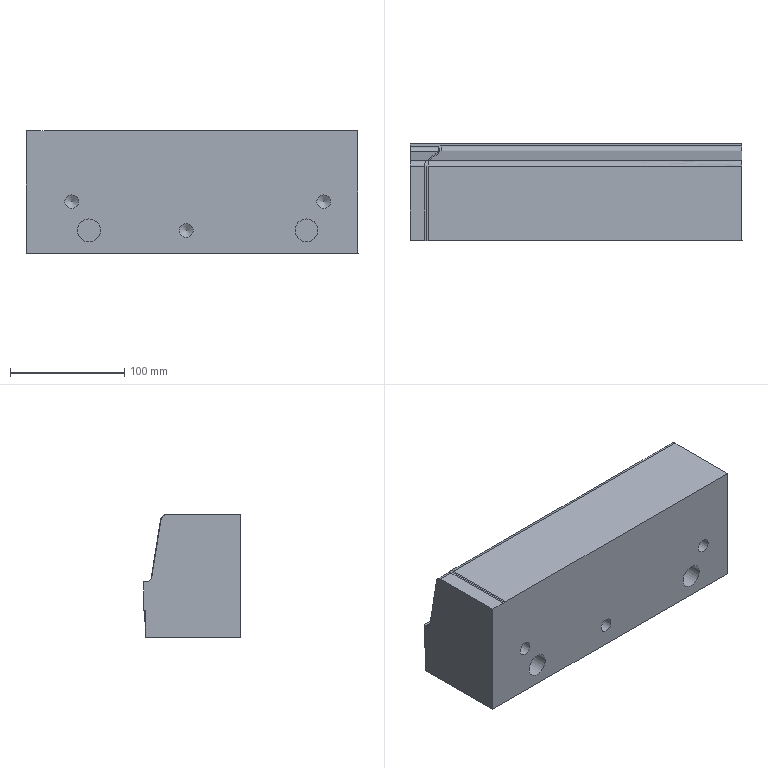Part | NX | features solid 2 | 1 solid | 33 faces | box 290 x 84.721 x 107.133 mm | volume 2405435 mm3 | plane 12 | cylinder 10 | spline 8 | cone 3 | commonest cylinder face diameters 12 x5 10 x3 20 x2
STEP:
#1=CARTESIAN_POINT('',(-215.,-160.,-50.));
#2=VERTEX_POINT('',#1);
#3=CARTESIAN_POINT('',(75.,-160.,-50.));
#4=VERTEX_POINT('',#3);
#5=CARTESIAN_POINT('',(-571.479,-160.,-50.));
#6=DIRECTION('',(1.,0.,0.));
#7=VECTOR('',#6,1000.);
#8=LINE('',#5,#7);
#9=EDGE_CURVE('',#2,#4,#8,.T.);
#10=ORIENTED_EDGE('',*,*,#9,.F.);
#11=CARTESIAN_POINT('',(-215.,-77.115,-50.));
#12=VERTEX_POINT('',#11);
#13=CARTESIAN_POINT('',(-215.,-74.471,-50.));
#14=DIRECTION('',(0.,1.,0.));
#15=VECTOR('',#14,1000.);
#16=LINE('',#13,#15);
#17=EDGE_CURVE('',#2,#12,#16,.T.);
#18=ORIENTED_EDGE('',*,*,#17,.T.);
#19=CARTESIAN_POINT('',(75.,-76.708,-50.));
#20=VERTEX_POINT('',#19);
#21=CARTESIAN_POINT('',(-215.,-77.115,-50.));
#22=CARTESIAN_POINT('',(-211.979,-77.116,-50.));
#23=CARTESIAN_POINT('',(-207.448,-77.118,-50.));
#24=CARTESIAN_POINT('',(-201.406,-77.119,-50.));
#25=CARTESIAN_POINT('',(-197.63,-77.126,-50.));
#26=CARTESIAN_POINT('',(-194.609,-77.116,-50.));
#27=CARTESIAN_POINT('',(-192.344,-77.15,-50.));
#28=CARTESIAN_POINT('',(-190.078,-77.04,-50.));
#29=CARTESIAN_POINT('',(-187.813,-76.65,-50.));
#30=CARTESIAN_POINT('',(-185.547,-76.717,-50.));
#31=CARTESIAN_POINT('',(-182.527,-76.699,-50.));
#32=CARTESIAN_POINT('',(-177.24,-76.699,-50.));
#33=CARTESIAN_POINT('',(-169.688,-76.703,-50.));
#34=CARTESIAN_POINT('',(-157.605,-76.713,-50.));
#35=CARTESIAN_POINT('',(-136.459,-76.708,-50.));
#36=CARTESIAN_POINT('',(-106.25,-76.699,-50.));
#37=CARTESIAN_POINT('',(-57.917,-76.699,-50.));
#38=CARTESIAN_POINT('',(2.5,-76.706,-50.));
#39=CARTESIAN_POINT('',(50.833,-76.708,-50.));
#40=CARTESIAN_POINT('',(75.,-76.708,-50.));
#41=B_SPLINE_CURVE_WITH_KNOTS('',3,(#21,#22,#23,#24,#25,#26,#27,#28,#29,#30,#31,#32,#33,#34,#35,#36,#37,#38,#39,#40),.UNSPECIFIED.,.F.,.F.,(4,1,1,1,1,1,1,1,1,1,1,1,1,1,1,1,1,4),(0.1494,0.1584,0.163,0.1675,0.1698,0.172,0.1743,0.1766,0.1788,0.1811,0.1856,0.1947,0.2037,0.2219,0.2581,0.2944,0.3669,0.4394),.UNSPECIFIED.);
#42=EDGE_CURVE('',#12,#20,#41,.T.);
#43=ORIENTED_EDGE('',*,*,#42,.T.);
#44=CARTESIAN_POINT('',(75.,-159.,-50.));
#45=DIRECTION('',(0.,1.,0.));
#46=VECTOR('',#45,1000.);
#47=LINE('',#44,#46);
#48=EDGE_CURVE('',#4,#20,#47,.T.);
#49=ORIENTED_EDGE('',*,*,#48,.F.);
#50=EDGE_LOOP('',(#10,#18,#43,#49));
#51=FACE_BOUND('',#50,.T.);
#52=CARTESIAN_POINT('',(-571.479,-74.471,-50.));
#53=DIRECTION('',(0.,0.,-1.));
#54=DIRECTION('',(-1.,0.,0.));
#55=AXIS2_PLACEMENT_3D('',#52,#53,#54);
#56=PLANE('',#55);
#57=ADVANCED_FACE('',(#51),#56,.T.);
#58=ORIENTED_EDGE('',*,*,#42,.F.);
#59=CARTESIAN_POINT('',(-215.,-76.915,-26.496));
#60=VERTEX_POINT('',#59);
#61=CARTESIAN_POINT('',(-215.,-77.015,-38.265));
#62=DIRECTION('',(0.,-0.008536,-1.));
#63=VECTOR('',#62,1000.);
#64=LINE('',#61,#63);
#65=EDGE_CURVE('',#12,#60,#64,.F.);
#66=ORIENTED_EDGE('',*,*,#65,.T.);
#67=CARTESIAN_POINT('',(75.,-76.507,-26.5));
#68=VERTEX_POINT('',#67);
#69=CARTESIAN_POINT('',(-215.,-76.915,-26.496));
#70=CARTESIAN_POINT('',(-211.979,-76.915,-26.496));
#71=CARTESIAN_POINT('',(-207.448,-76.918,-26.496));
#72=CARTESIAN_POINT('',(-201.406,-76.918,-26.496));
#73=CARTESIAN_POINT('',(-197.63,-76.925,-26.496));
#74=CARTESIAN_POINT('',(-194.609,-76.916,-26.496));
#75=CARTESIAN_POINT('',(-192.344,-76.949,-26.496));
#76=CARTESIAN_POINT('',(-190.078,-76.839,-26.497));
#77=CARTESIAN_POINT('',(-187.813,-76.449,-26.5));
#78=CARTESIAN_POINT('',(-185.547,-76.516,-26.499));
#79=CARTESIAN_POINT('',(-182.527,-76.499,-26.5));
#80=CARTESIAN_POINT('',(-177.24,-76.499,-26.5));
#81=CARTESIAN_POINT('',(-169.688,-76.502,-26.5));
#82=CARTESIAN_POINT('',(-157.605,-76.512,-26.5));
#83=CARTESIAN_POINT('',(-136.459,-76.507,-26.5));
#84=CARTESIAN_POINT('',(-106.25,-76.499,-26.5));
#85=CARTESIAN_POINT('',(-57.917,-76.498,-26.5));
#86=CARTESIAN_POINT('',(2.5,-76.505,-26.5));
#87=CARTESIAN_POINT('',(50.833,-76.507,-26.5));
#88=CARTESIAN_POINT('',(75.,-76.507,-26.5));
#89=B_SPLINE_CURVE_WITH_KNOTS('',3,(#69,#70,#71,#72,#73,#74,#75,#76,#77,#78,#79,#80,#81,#82,#83,#84,#85,#86,#87,#88),.UNSPECIFIED.,.F.,.F.,(4,1,1,1,1,1,1,1,1,1,1,1,1,1,1,1,1,4),(0.1353,0.1444,0.1489,0.1535,0.1557,0.158,0.1603,0.1625,0.1648,0.1671,0.1716,0.1807,0.1897,0.2078,0.2441,0.2803,0.3528,0.4253),.UNSPECIFIED.);
#90=EDGE_CURVE('',#60,#68,#89,.T.);
#91=ORIENTED_EDGE('',*,*,#90,.T.);
#92=CARTESIAN_POINT('',(75.,-76.608,-38.267));
#93=DIRECTION('',(0.,-0.008536,-1.));
#94=VECTOR('',#93,1000.);
#95=LINE('',#92,#94);
#96=EDGE_CURVE('',#20,#68,#95,.F.);
#97=ORIENTED_EDGE('',*,*,#96,.F.);
#98=EDGE_LOOP('',(#58,#66,#91,#97));
#99=FACE_BOUND('',#98,.T.);
#100=CARTESIAN_POINT('',(-215.,-76.915,-26.496));
#101=CARTESIAN_POINT('',(-215.,-77.117,-50.141));
#102=CARTESIAN_POINT('',(-211.979,-76.915,-26.496));
#103=CARTESIAN_POINT('',(-211.979,-77.117,-50.141));
#104=CARTESIAN_POINT('',(-207.449,-76.918,-26.496));
#105=CARTESIAN_POINT('',(-207.449,-77.12,-50.141));
#106=CARTESIAN_POINT('',(-201.403,-76.918,-26.496));
#107=CARTESIAN_POINT('',(-201.403,-77.12,-50.141));
#108=CARTESIAN_POINT('',(-197.637,-76.926,-26.496));
#109=CARTESIAN_POINT('',(-197.637,-77.128,-50.141));
#110=CARTESIAN_POINT('',(-194.595,-76.914,-26.496));
#111=CARTESIAN_POINT('',(-194.595,-77.116,-50.141));
#112=CARTESIAN_POINT('',(-192.394,-76.956,-26.496));
#113=CARTESIAN_POINT('',(-192.394,-77.158,-50.141));
#114=CARTESIAN_POINT('',(-189.892,-76.814,-26.497));
#115=CARTESIAN_POINT('',(-189.892,-77.016,-50.142));
#116=CARTESIAN_POINT('',(-187.778,-76.451,-26.5));
#117=CARTESIAN_POINT('',(-187.778,-76.653,-50.145));
#118=CARTESIAN_POINT('',(-185.598,-76.515,-26.499));
#119=CARTESIAN_POINT('',(-185.598,-76.717,-50.145));
#120=CARTESIAN_POINT('',(-182.526,-76.499,-26.5));
#121=CARTESIAN_POINT('',(-182.526,-76.701,-50.145));
#122=CARTESIAN_POINT('',(-177.274,-76.498,-26.5));
#123=CARTESIAN_POINT('',(-177.274,-76.7,-50.145));
#124=CARTESIAN_POINT('',(-169.704,-76.502,-26.5));
#125=CARTESIAN_POINT('',(-169.704,-76.704,-50.145));
#126=CARTESIAN_POINT('',(-157.625,-76.512,-26.5));
#127=CARTESIAN_POINT('',(-157.625,-76.714,-50.145));
#128=CARTESIAN_POINT('',(-136.473,-76.507,-26.5));
#129=CARTESIAN_POINT('',(-136.473,-76.709,-50.145));
#130=CARTESIAN_POINT('',(-106.265,-76.499,-26.5));
#131=CARTESIAN_POINT('',(-106.265,-76.701,-50.145));
#132=CARTESIAN_POINT('',(-57.927,-76.498,-26.5));
#133=CARTESIAN_POINT('',(-57.927,-76.7,-50.145));
#134=CARTESIAN_POINT('',(2.494,-76.505,-26.5));
#135=CARTESIAN_POINT('',(2.494,-76.707,-50.145));
#136=CARTESIAN_POINT('',(50.831,-76.507,-26.5));
#137=CARTESIAN_POINT('',(50.831,-76.709,-50.145));
#138=CARTESIAN_POINT('',(75.,-76.507,-26.5));
#139=CARTESIAN_POINT('',(75.,-76.709,-50.145));
#140=B_SPLINE_SURFACE_WITH_KNOTS('',3,1,((#100,#101),(#102,#103),(#104,#105),(#106,#107),(#108,#109),(#110,#111),(#112,#113),(#114,#115),(#116,#117),(#118,#119),(#120,#121),(#122,#123),(#124,#125),(#126,#127),(#128,#129),(#130,#131),(#132,#133),(#134,#135),(#136,#137),(#138,#139)),.SURF_OF_LINEAR_EXTRUSION.,.F.,.F.,.F.,(4,1,1,1,1,1,1,1,1,1,1,1,1,1,1,1,1,4),(2,2),(0.3592,0.3659,0.3692,0.3725,0.3742,0.3758,0.3775,0.3791,0.3808,0.3825,0.3858,0.3924,0.3991,0.4123,0.4389,0.4654,0.5185,0.5716),(0.,1.),.UNSPECIFIED.);
#141=ADVANCED_FACE('',(#99),#140,.T.);
#142=ORIENTED_EDGE('',*,*,#96,.T.);
#143=CARTESIAN_POINT('',(75.,-75.294,-26.51));
#144=VERTEX_POINT('',#143);
#145=CARTESIAN_POINT('',(75.,-75.914,-26.505));
#146=DIRECTION('',(0.,-1.,0.008536));
#147=VECTOR('',#146,1000.);
#148=LINE('',#145,#147);
#149=EDGE_CURVE('',#144,#68,#148,.T.);
#150=ORIENTED_EDGE('',*,*,#149,.F.);
#151=CARTESIAN_POINT('',(75.,-75.294,-1.509));
#152=VERTEX_POINT('',#151);
#153=CARTESIAN_POINT('',(75.,-75.294,-14.008));
#154=DIRECTION('',(0.,0.,-1.));
#155=VECTOR('',#154,1000.);
#156=LINE('',#153,#155);
#157=EDGE_CURVE('',#152,#144,#156,.T.);
#158=ORIENTED_EDGE('',*,*,#157,.F.);
#159=CARTESIAN_POINT('',(75.,-77.294,-1.492));
#160=VERTEX_POINT('',#159);
#161=CARTESIAN_POINT('',(75.,47.797,-2.56));
#162=DIRECTION('',(0.,1.,-0.008536));
#163=VECTOR('',#162,1000.);
#164=LINE('',#161,#163);
#165=EDGE_CURVE('',#160,#152,#164,.T.);
#166=ORIENTED_EDGE('',*,*,#165,.F.);
#167=CARTESIAN_POINT('',(75.,-82.189,2.72));
#168=VERTEX_POINT('',#167);
#169=CARTESIAN_POINT('',(75.,-77.252,3.508));
#170=DIRECTION('',(-1.,0.,0.));
#171=DIRECTION('',(0.,0.,1.));
#172=AXIS2_PLACEMENT_3D('',#169,#170,#171);
#173=CIRCLE('',#172,5.);
#174=EDGE_CURVE('',#168,#160,#173,.F.);
#175=ORIENTED_EDGE('',*,*,#174,.F.);
#176=CARTESIAN_POINT('',(75.,-90.197,52.92));
#177=VERTEX_POINT('',#176);
#178=CARTESIAN_POINT('',(75.,-86.499,29.736));
#179=DIRECTION('',(0.,0.1575,-0.9875));
#180=VECTOR('',#179,1000.);
#181=LINE('',#178,#180);
#182=EDGE_CURVE('',#177,#168,#181,.T.);
#183=ORIENTED_EDGE('',*,*,#182,.F.);
#184=CARTESIAN_POINT('',(75.,-95.134,57.133));
#185=VERTEX_POINT('',#184);
#186=CARTESIAN_POINT('',(75.,-95.134,52.133));
#187=DIRECTION('',(-1.,0.,0.));
#188=DIRECTION('',(0.,0.,1.));
#189=AXIS2_PLACEMENT_3D('',#186,#187,#188);
#190=CIRCLE('',#189,5.);
#191=EDGE_CURVE('',#177,#185,#190,.F.);
#192=ORIENTED_EDGE('',*,*,#191,.T.);
#193=CARTESIAN_POINT('',(75.,-160.,57.133));
#194=VERTEX_POINT('',#193);
#195=CARTESIAN_POINT('',(75.,-90.869,57.133));
#196=DIRECTION('',(0.,-1.,0.));
#197=VECTOR('',#196,1000.);
#198=LINE('',#195,#197);
#199=EDGE_CURVE('',#185,#194,#198,.T.);
#200=ORIENTED_EDGE('',*,*,#199,.T.);
#201=CARTESIAN_POINT('',(75.,-160.,200.));
#202=DIRECTION('',(0.,0.,1.));
#203=VECTOR('',#202,1000.);
#204=LINE('',#201,#203);
#205=EDGE_CURVE('',#4,#194,#204,.T.);
#206=ORIENTED_EDGE('',*,*,#205,.F.);
#207=ORIENTED_EDGE('',*,*,#48,.T.);
#208=EDGE_LOOP('',(#142,#150,#158,#166,#175,#183,#192,#200,#206,#207));
#209=FACE_BOUND('',#208,.T.);
#210=CARTESIAN_POINT('',(75.,361.,0.));
#211=DIRECTION('',(-1.,0.,0.));
#212=DIRECTION('',(0.,0.,1.));
#213=AXIS2_PLACEMENT_3D('',#210,#211,#212);
#214=PLANE('',#213);
#215=ADVANCED_FACE('',(#209),#214,.F.);
#216=CARTESIAN_POINT('',(-215.,-160.,57.07));
#217=VERTEX_POINT('',#216);
#218=CARTESIAN_POINT('',(-215.,-160.,200.));
#219=DIRECTION('',(0.,0.,1.));
#220=VECTOR('',#219,1000.);
#221=LINE('',#218,#220);
#222=EDGE_CURVE('',#2,#217,#221,.T.);
#223=ORIENTED_EDGE('',*,*,#222,.F.);
#224=ORIENTED_EDGE('',*,*,#9,.T.);
#225=ORIENTED_EDGE('',*,*,#205,.T.);
#226=CARTESIAN_POINT('',(-198.963,-160.,57.133));
#227=VERTEX_POINT('',#226);
#228=CARTESIAN_POINT('',(-705.,-160.,57.133));
#229=DIRECTION('',(1.,0.,0.));
#230=VECTOR('',#229,1000.);
#231=LINE('',#228,#230);
#232=EDGE_CURVE('',#227,#194,#231,.T.);
#233=ORIENTED_EDGE('',*,*,#232,.F.);
#234=CARTESIAN_POINT('',(-200.536,-160.,57.112));
#235=VERTEX_POINT('',#234);
#236=CARTESIAN_POINT('',(-703.043,-160.,50.532));
#237=DIRECTION('',(0.9999,0.,0.01309));
#238=VECTOR('',#237,1000.);
#239=LINE('',#236,#238);
#240=EDGE_CURVE('',#235,#227,#239,.T.);
#241=ORIENTED_EDGE('',*,*,#240,.F.);
#242=CARTESIAN_POINT('',(-202.104,-160.,57.07));
#243=VERTEX_POINT('',#242);
#244=CARTESIAN_POINT('',(-200.536,-160.,57.112));
#245=CARTESIAN_POINT('',(-201.059,-160.,57.095));
#246=CARTESIAN_POINT('',(-201.581,-160.,57.081));
#247=CARTESIAN_POINT('',(-202.104,-160.,57.075));
#248=B_SPLINE_CURVE_WITH_KNOTS('',3,(#244,#245,#246,#247),.UNSPECIFIED.,.F.,.F.,(4,4),(0.006154,0.007723),.UNSPECIFIED.);
#249=EDGE_CURVE('',#243,#235,#248,.F.);
#250=ORIENTED_EDGE('',*,*,#249,.F.);
#251=CARTESIAN_POINT('',(-705.,-160.,57.07));
#252=DIRECTION('',(-1.,0.,0.));
#253=VECTOR('',#252,1000.);
#254=LINE('',#251,#253);
#255=EDGE_CURVE('',#243,#217,#254,.T.);
#256=ORIENTED_EDGE('',*,*,#255,.T.);
#257=EDGE_LOOP('',(#223,#224,#225,#233,#241,#250,#256));
#258=FACE_BOUND('',#257,.T.);
#259=CARTESIAN_POINT('',(45.,-160.,1.));
#260=VERTEX_POINT('',#259);
#261=CARTESIAN_POINT('',(45.,-160.,-5.));
#262=DIRECTION('',(0.,1.,0.));
#263=DIRECTION('',(0.,0.,1.));
#264=AXIS2_PLACEMENT_3D('',#261,#262,#263);
#265=CIRCLE('',#264,6.);
#266=EDGE_CURVE('',#260,#260,#265,.T.);
#267=ORIENTED_EDGE('',*,*,#266,.T.);
#268=EDGE_LOOP('',(#267));
#269=FACE_BOUND('',#268,.T.);
#270=CARTESIAN_POINT('',(-75.,-160.,-24.));
#271=VERTEX_POINT('',#270);
#272=CARTESIAN_POINT('',(-75.,-160.,-30.));
#273=DIRECTION('',(0.,1.,0.));
#274=DIRECTION('',(0.,0.,1.));
#275=AXIS2_PLACEMENT_3D('',#272,#273,#274);
#276=CIRCLE('',#275,6.);
#277=EDGE_CURVE('',#271,#271,#276,.T.);
#278=ORIENTED_EDGE('',*,*,#277,.T.);
#279=EDGE_LOOP('',(#278));
#280=FACE_BOUND('',#279,.T.);
#281=CARTESIAN_POINT('',(-175.,-160.,1.));
#282=VERTEX_POINT('',#281);
#283=CARTESIAN_POINT('',(-175.,-160.,-5.));
#284=DIRECTION('',(0.,1.,0.));
#285=DIRECTION('',(0.,0.,1.));
#286=AXIS2_PLACEMENT_3D('',#283,#284,#285);
#287=CIRCLE('',#286,6.);
#288=EDGE_CURVE('',#282,#282,#287,.T.);
#289=ORIENTED_EDGE('',*,*,#288,.T.);
#290=EDGE_LOOP('',(#289));
#291=FACE_BOUND('',#290,.T.);
#292=CARTESIAN_POINT('',(30.,-160.,-20.));
#293=VERTEX_POINT('',#292);
#294=CARTESIAN_POINT('',(30.,-160.,-30.));
#295=DIRECTION('',(0.,1.,0.));
#296=DIRECTION('',(0.,0.,1.));
#297=AXIS2_PLACEMENT_3D('',#294,#295,#296);
#298=CIRCLE('',#297,10.);
#299=EDGE_CURVE('',#293,#293,#298,.T.);
#300=ORIENTED_EDGE('',*,*,#299,.T.);
#301=EDGE_LOOP('',(#300));
#302=FACE_BOUND('',#301,.T.);
#303=CARTESIAN_POINT('',(-160.,-160.,-20.));
#304=VERTEX_POINT('',#303);
#305=CARTESIAN_POINT('',(-160.,-160.,-30.));
#306=DIRECTION('',(0.,1.,0.));
#307=DIRECTION('',(0.,0.,1.));
#308=AXIS2_PLACEMENT_3D('',#305,#306,#307);
#309=CIRCLE('',#308,10.);
#310=EDGE_CURVE('',#304,#304,#309,.T.);
#311=ORIENTED_EDGE('',*,*,#310,.T.);
#312=EDGE_LOOP('',(#311));
#313=FACE_BOUND('',#312,.T.);
#314=CARTESIAN_POINT('',(-705.,-160.,200.));
#315=DIRECTION('',(0.,1.,0.));
#316=DIRECTION('',(0.,0.,1.));
#317=AXIS2_PLACEMENT_3D('',#314,#315,#316);
#318=PLANE('',#317);
#319=ADVANCED_FACE('',(#258,#269,#280,#291,#302,#313),#318,.F.);
#320=CARTESIAN_POINT('',(-215.,-75.704,-26.506));
#321=VERTEX_POINT('',#320);
#322=CARTESIAN_POINT('',(-215.,-75.914,-26.505));
#323=DIRECTION('',(0.,-1.,0.008536));
#324=VECTOR('',#323,1000.);
#325=LINE('',#322,#324);
#326=EDGE_CURVE('',#321,#60,#325,.T.);
#327=ORIENTED_EDGE('',*,*,#326,.T.);
#328=ORIENTED_EDGE('',*,*,#65,.F.);
#329=ORIENTED_EDGE('',*,*,#17,.F.);
#330=ORIENTED_EDGE('',*,*,#222,.T.);
#331=CARTESIAN_POINT('',(-215.,-95.529,57.07));
#332=VERTEX_POINT('',#331);
#333=CARTESIAN_POINT('',(-215.,-391.264,57.07));
#334=DIRECTION('',(0.,1.,0.));
#335=VECTOR('',#334,1000.);
#336=LINE('',#333,#335);
#337=EDGE_CURVE('',#217,#332,#336,.T.);
#338=ORIENTED_EDGE('',*,*,#337,.T.);
#339=CARTESIAN_POINT('',(-215.,-90.592,52.857));
#340=VERTEX_POINT('',#339);
#341=CARTESIAN_POINT('',(-215.,-95.529,52.07));
#342=DIRECTION('',(-1.,0.,0.));
#343=DIRECTION('',(0.,0.,1.));
#344=AXIS2_PLACEMENT_3D('',#341,#342,#343);
#345=CIRCLE('',#344,5.);
#346=EDGE_CURVE('',#340,#332,#345,.F.);
#347=ORIENTED_EDGE('',*,*,#346,.F.);
#348=CARTESIAN_POINT('',(-215.,-82.595,2.724));
#349=VERTEX_POINT('',#348);
#350=CARTESIAN_POINT('',(-215.,-78.399,-23.581));
#351=DIRECTION('',(0.,0.1575,-0.9875));
#352=VECTOR('',#351,1000.);
#353=LINE('',#350,#352);
#354=EDGE_CURVE('',#340,#349,#353,.T.);
#355=ORIENTED_EDGE('',*,*,#354,.T.);
#356=CARTESIAN_POINT('',(-215.,-77.7,-1.488));
#357=VERTEX_POINT('',#356);
#358=CARTESIAN_POINT('',(-215.,-77.657,3.511));
#359=DIRECTION('',(-1.,0.,0.));
#360=DIRECTION('',(0.,0.,1.));
#361=AXIS2_PLACEMENT_3D('',#358,#359,#360);
#362=CIRCLE('',#361,5.);
#363=EDGE_CURVE('',#349,#357,#362,.F.);
#364=ORIENTED_EDGE('',*,*,#363,.T.);
#365=CARTESIAN_POINT('',(-215.,-75.704,-1.506));
#366=VERTEX_POINT('',#365);
#367=CARTESIAN_POINT('',(-215.,47.797,-2.56));
#368=DIRECTION('',(0.,1.,-0.008536));
#369=VECTOR('',#368,1000.);
#370=LINE('',#367,#369);
#371=EDGE_CURVE('',#357,#366,#370,.T.);
#372=ORIENTED_EDGE('',*,*,#371,.T.);
#373=CARTESIAN_POINT('',(-215.,-75.704,-14.008));
#374=DIRECTION('',(0.,0.,-1.));
#375=VECTOR('',#374,1000.);
#376=LINE('',#373,#375);
#377=EDGE_CURVE('',#366,#321,#376,.T.);
#378=ORIENTED_EDGE('',*,*,#377,.T.);
#379=EDGE_LOOP('',(#327,#328,#329,#330,#338,#347,#355,#364,#372,#378));
#380=FACE_BOUND('',#379,.T.);
#381=CARTESIAN_POINT('',(-215.,361.,0.));
#382=DIRECTION('',(-1.,0.,0.));
#383=DIRECTION('',(0.,0.,1.));
#384=AXIS2_PLACEMENT_3D('',#381,#382,#383);
#385=PLANE('',#384);
#386=ADVANCED_FACE('',(#380),#385,.T.);
#387=CARTESIAN_POINT('',(-199.628,-90.395,52.891));
#388=VERTEX_POINT('',#387);
#389=CARTESIAN_POINT('',(-198.056,-90.197,52.92));
#390=VERTEX_POINT('',#389);
#391=CARTESIAN_POINT('',(-199.628,-90.395,52.894));
#392=CARTESIAN_POINT('',(-199.206,-90.287,52.907));
#393=CARTESIAN_POINT('',(-198.679,-90.197,52.92));
#394=CARTESIAN_POINT('',(-198.056,-90.197,52.92));
#395=B_SPLINE_CURVE_WITH_KNOTS('',3,(#391,#392,#393,#394),.UNSPECIFIED.,.F.,.F.,(4,4),(0.6644,1.),.UNSPECIFIED.);
#396=EDGE_CURVE('',#388,#390,#395,.T.);
#397=ORIENTED_EDGE('',*,*,#396,.T.);
#398=CARTESIAN_POINT('',(-196.309,-88.902,44.803));
#399=VERTEX_POINT('',#398);
#400=CARTESIAN_POINT('',(-196.309,-88.902,44.803));
#401=CARTESIAN_POINT('',(-196.892,-89.333,47.509));
#402=CARTESIAN_POINT('',(-197.474,-89.765,50.215));
#403=CARTESIAN_POINT('',(-198.056,-90.197,52.92));
#404=B_SPLINE_CURVE_WITH_KNOTS('',3,(#400,#401,#402,#403),.UNSPECIFIED.,.F.,.F.,(4,4),(0.,1.),.UNSPECIFIED.);
#405=EDGE_CURVE('',#399,#390,#404,.T.);
#406=ORIENTED_EDGE('',*,*,#405,.F.);
#407=CARTESIAN_POINT('',(-194.188,-87.33,34.95));
#408=VERTEX_POINT('',#407);
#409=CARTESIAN_POINT('',(-194.188,-87.33,34.95));
#410=CARTESIAN_POINT('',(-194.895,-87.854,38.234));
#411=CARTESIAN_POINT('',(-195.602,-88.378,41.518));
#412=CARTESIAN_POINT('',(-196.309,-88.902,44.803));
#413=B_SPLINE_CURVE_WITH_KNOTS('',3,(#409,#410,#411,#412),.UNSPECIFIED.,.F.,.F.,(4,4),(0.,1.),.UNSPECIFIED.);
#414=EDGE_CURVE('',#408,#399,#413,.T.);
#415=ORIENTED_EDGE('',*,*,#414,.F.);
#416=CARTESIAN_POINT('',(-187.251,-82.189,2.72));
#417=VERTEX_POINT('',#416);
#418=CARTESIAN_POINT('',(-187.251,-82.189,2.72));
#419=CARTESIAN_POINT('',(-189.564,-83.903,13.463));
#420=CARTESIAN_POINT('',(-191.876,-85.617,24.207));
#421=CARTESIAN_POINT('',(-194.188,-87.33,34.95));
#422=B_SPLINE_CURVE_WITH_KNOTS('',3,(#418,#419,#420,#421),.UNSPECIFIED.,.F.,.F.,(4,4),(0.,1.),.UNSPECIFIED.);
#423=EDGE_CURVE('',#417,#408,#422,.T.);
#424=ORIENTED_EDGE('',*,*,#423,.F.);
#425=CARTESIAN_POINT('',(-188.891,-82.438,3.013));
#426=VERTEX_POINT('',#425);
#427=CARTESIAN_POINT('',(-188.891,-82.438,3.013));
#428=CARTESIAN_POINT('',(-188.315,-82.277,2.9));
#429=CARTESIAN_POINT('',(-187.761,-82.202,2.803));
#430=CARTESIAN_POINT('',(-187.251,-82.189,2.72));
#431=B_SPLINE_CURVE_WITH_KNOTS('',3,(#427,#428,#429,#430),.UNSPECIFIED.,.F.,.F.,(4,4),(0.,1.),.UNSPECIFIED.);
#432=EDGE_CURVE('',#417,#426,#431,.F.);
#433=ORIENTED_EDGE('',*,*,#432,.T.);
#434=CARTESIAN_POINT('',(-195.756,-87.526,34.905));
#435=VERTEX_POINT('',#434);
#436=CARTESIAN_POINT('',(-195.756,-87.526,34.905));
#437=CARTESIAN_POINT('',(-193.468,-85.83,24.274));
#438=CARTESIAN_POINT('',(-191.18,-84.134,13.643));
#439=CARTESIAN_POINT('',(-188.891,-82.438,3.013));
#440=B_SPLINE_CURVE_WITH_KNOTS('',3,(#436,#437,#438,#439),.UNSPECIFIED.,.F.,.F.,(4,4),(0.,1.),.UNSPECIFIED.);
#441=EDGE_CURVE('',#426,#435,#440,.F.);
#442=ORIENTED_EDGE('',*,*,#441,.T.);
#443=CARTESIAN_POINT('',(-197.877,-89.097,44.758));
#444=VERTEX_POINT('',#443);
#445=CARTESIAN_POINT('',(-190.129,-83.356,8.763));
#446=DIRECTION('',(-0.2079,-0.1541,0.9659));
#447=VECTOR('',#446,1000.);
#448=LINE('',#445,#447);
#449=EDGE_CURVE('',#435,#444,#448,.T.);
#450=ORIENTED_EDGE('',*,*,#449,.T.);
#451=CARTESIAN_POINT('',(-199.628,-90.395,52.894));
#452=CARTESIAN_POINT('',(-199.044,-89.962,50.182));
#453=CARTESIAN_POINT('',(-198.461,-89.53,47.47));
#454=CARTESIAN_POINT('',(-197.877,-89.097,44.758));
#455=B_SPLINE_CURVE_WITH_KNOTS('',3,(#451,#452,#453,#454),.UNSPECIFIED.,.F.,.F.,(4,4),(0.,1.),.UNSPECIFIED.);
#456=EDGE_CURVE('',#444,#388,#455,.F.);
#457=ORIENTED_EDGE('',*,*,#456,.T.);
#458=EDGE_LOOP('',(#397,#406,#415,#424,#433,#442,#450,#457));
#459=FACE_BOUND('',#458,.T.);
#460=CARTESIAN_POINT('',(-188.626,-89.134,8.164));
#461=DIRECTION('',(-0.2079,-0.1541,0.9659));
#462=DIRECTION('',(0.9781,-0.03275,0.2053));
#463=AXIS2_PLACEMENT_3D('',#460,#461,#462);
#464=CYLINDRICAL_SURFACE('',#463,6.);
#465=ADVANCED_FACE('',(#459),#464,.T.);
#466=ORIENTED_EDGE('',*,*,#191,.F.);
#467=CARTESIAN_POINT('',(-198.056,-90.197,52.92));
#468=CARTESIAN_POINT('',(-107.038,-90.197,52.92));
#469=CARTESIAN_POINT('',(-16.019,-90.197,52.92));
#470=CARTESIAN_POINT('',(75.,-90.197,52.92));
#471=B_SPLINE_CURVE_WITH_KNOTS('',3,(#467,#468,#469,#470),.UNSPECIFIED.,.F.,.F.,(4,4),(0.,0.2731),.UNSPECIFIED.);
#472=EDGE_CURVE('',#390,#177,#471,.T.);
#473=ORIENTED_EDGE('',*,*,#472,.F.);
#474=CARTESIAN_POINT('',(-198.963,-95.134,57.132));
#475=VERTEX_POINT('',#474);
#476=CARTESIAN_POINT('',(-198.963,-95.133,57.132));
#477=CARTESIAN_POINT('',(-198.958,-93.944,57.111));
#478=CARTESIAN_POINT('',(-198.774,-91.575,56.253));
#479=CARTESIAN_POINT('',(-198.303,-90.389,54.067));
#480=CARTESIAN_POINT('',(-198.056,-90.197,52.92));
#481=B_SPLINE_CURVE_WITH_KNOTS('',3,(#476,#477,#478,#479,#480),.UNSPECIFIED.,.F.,.F.,(4,1,4),(0.,0.5,1.),.UNSPECIFIED.);
#482=EDGE_CURVE('',#475,#390,#481,.T.);
#483=ORIENTED_EDGE('',*,*,#482,.F.);
#484=CARTESIAN_POINT('',(75.,-95.134,57.133));
#485=CARTESIAN_POINT('',(-16.321,-95.134,57.133));
#486=CARTESIAN_POINT('',(-107.642,-95.134,57.133));
#487=CARTESIAN_POINT('',(-198.963,-95.134,57.133));
#488=B_SPLINE_CURVE_WITH_KNOTS('',3,(#484,#485,#486,#487),.UNSPECIFIED.,.F.,.F.,(4,4),(0.6686,0.9426),.UNSPECIFIED.);
#489=EDGE_CURVE('',#185,#475,#488,.T.);
#490=ORIENTED_EDGE('',*,*,#489,.F.);
#491=EDGE_LOOP('',(#466,#473,#483,#490));
#492=FACE_BOUND('',#491,.T.);
#493=CARTESIAN_POINT('',(75.,-90.197,52.92));
#494=CARTESIAN_POINT('',(75.,-90.869,57.133));
#495=CARTESIAN_POINT('',(75.,-95.134,57.133));
#496=CARTESIAN_POINT('',(-16.869,-90.197,52.92));
#497=CARTESIAN_POINT('',(-16.869,-90.869,57.133));
#498=CARTESIAN_POINT('',(-16.869,-95.134,57.133));
#499=CARTESIAN_POINT('',(-108.738,-90.197,52.92));
#500=CARTESIAN_POINT('',(-108.738,-90.869,57.133));
#501=CARTESIAN_POINT('',(-108.738,-95.134,57.133));
#502=CARTESIAN_POINT('',(-200.607,-90.197,52.92));
#503=CARTESIAN_POINT('',(-200.607,-90.869,57.133));
#504=CARTESIAN_POINT('',(-200.607,-95.134,57.133));
#505=(BOUNDED_SURFACE()B_SPLINE_SURFACE(3,2,((#493,#494,#495),(#496,#497,#498),(#499,#500,#501),(#502,#503,#504)),.UNSPECIFIED.,.F.,.F.,.F.)B_SPLINE_SURFACE_WITH_KNOTS((4,4),(3,3),(0.7843,1.06),(0.,1.),.PIECEWISE_BEZIER_KNOTS.)GEOMETRIC_REPRESENTATION_ITEM()RATIONAL_B_SPLINE_SURFACE(((1.,0.7608,1.),(1.,0.7608,1.),(1.,0.7608,1.),(1.,0.7608,1.)))REPRESENTATION_ITEM('')SURFACE());
#506=ADVANCED_FACE('',(#492),#505,.T.);
#507=ORIENTED_EDGE('',*,*,#472,.T.);
#508=ORIENTED_EDGE('',*,*,#182,.T.);
#509=CARTESIAN_POINT('',(-187.251,-82.189,2.72));
#510=CARTESIAN_POINT('',(-99.834,-82.189,2.72));
#511=CARTESIAN_POINT('',(-12.417,-82.189,2.72));
#512=CARTESIAN_POINT('',(75.,-82.189,2.72));
#513=B_SPLINE_CURVE_WITH_KNOTS('',3,(#509,#510,#511,#512),.UNSPECIFIED.,.F.,.F.,(4,4),(0.,0.3113),.UNSPECIFIED.);
#514=EDGE_CURVE('',#417,#168,#513,.T.);
#515=ORIENTED_EDGE('',*,*,#514,.F.);
#516=ORIENTED_EDGE('',*,*,#423,.T.);
#517=ORIENTED_EDGE('',*,*,#414,.T.);
#518=ORIENTED_EDGE('',*,*,#405,.T.);
#519=EDGE_LOOP('',(#507,#508,#515,#516,#517,#518));
#520=FACE_BOUND('',#519,.T.);
#521=CARTESIAN_POINT('',(808.196,-81.695,-0.3814));
#522=CARTESIAN_POINT('',(-199.284,-81.695,-0.3814));
#523=CARTESIAN_POINT('',(808.196,-91.303,59.853));
#524=CARTESIAN_POINT('',(-199.284,-91.303,59.853));
#525=B_SPLINE_SURFACE_WITH_KNOTS('',1,1,((#521,#522),(#523,#524)),.PLANE_SURF.,.F.,.F.,.F.,(2,2),(2,2),(-0.06964,1.283),(-0.1722,1.),.UNSPECIFIED.);
#526=ADVANCED_FACE('',(#520),#525,.F.);
#527=CARTESIAN_POINT('',(-202.105,-95.529,57.073));
#528=VERTEX_POINT('',#527);
#529=CARTESIAN_POINT('',(-200.536,-95.332,57.107));
#530=VERTEX_POINT('',#529);
#531=CARTESIAN_POINT('',(-202.104,-95.529,57.075));
#532=CARTESIAN_POINT('',(-201.578,-95.529,57.081));
#533=CARTESIAN_POINT('',(-201.072,-95.436,57.094));
#534=CARTESIAN_POINT('',(-200.536,-95.332,57.112));
#535=B_SPLINE_CURVE_WITH_KNOTS('',3,(#531,#532,#533,#534),.UNSPECIFIED.,.F.,.F.,(4,4),(0.,0.9789),.UNSPECIFIED.);
#536=EDGE_CURVE('',#528,#530,#535,.T.);
#537=ORIENTED_EDGE('',*,*,#536,.T.);
#538=CARTESIAN_POINT('',(-200.536,-95.332,57.112));
#539=CARTESIAN_POINT('',(-200.011,-95.266,57.119));
#540=CARTESIAN_POINT('',(-199.487,-95.199,57.126));
#541=CARTESIAN_POINT('',(-198.963,-95.133,57.133));
#542=B_SPLINE_CURVE_WITH_KNOTS('',3,(#538,#539,#540,#541),.UNSPECIFIED.,.F.,.F.,(4,4),(0.,1.),.UNSPECIFIED.);
#543=EDGE_CURVE('',#530,#475,#542,.T.);
#544=ORIENTED_EDGE('',*,*,#543,.T.);
#545=ORIENTED_EDGE('',*,*,#482,.T.);
#546=ORIENTED_EDGE('',*,*,#396,.F.);
#547=CARTESIAN_POINT('',(-201.198,-90.592,52.857));
#548=VERTEX_POINT('',#547);
#549=CARTESIAN_POINT('',(-201.198,-90.592,52.857));
#550=CARTESIAN_POINT('',(-200.668,-90.592,52.859));
#551=CARTESIAN_POINT('',(-200.139,-90.525,52.87));
#552=CARTESIAN_POINT('',(-199.627,-90.394,52.889));
#553=B_SPLINE_CURVE_WITH_KNOTS('',3,(#549,#550,#551,#552),.UNSPECIFIED.,.F.,.F.,(4,4),(0.,0.9602),.UNSPECIFIED.);
#554=EDGE_CURVE('',#548,#388,#553,.T.);
#555=ORIENTED_EDGE('',*,*,#554,.F.);
#556=CARTESIAN_POINT('',(-201.198,-90.592,52.857));
#557=CARTESIAN_POINT('',(-201.5,-90.816,54.262));
#558=CARTESIAN_POINT('',(-201.953,-92.438,56.537));
#559=CARTESIAN_POINT('',(-202.104,-94.597,57.07));
#560=CARTESIAN_POINT('',(-202.104,-95.529,57.07));
#561=B_SPLINE_CURVE_WITH_KNOTS('',3,(#556,#557,#558,#559,#560),.UNSPECIFIED.,.F.,.F.,(4,1,4),(0.,0.5,1.),.UNSPECIFIED.);
#562=EDGE_CURVE('',#528,#548,#561,.F.);
#563=ORIENTED_EDGE('',*,*,#562,.F.);
#564=EDGE_LOOP('',(#537,#544,#545,#546,#555,#563));
#565=FACE_BOUND('',#564,.T.);
#566=CARTESIAN_POINT('',(-202.104,-95.53,57.07));
#567=CARTESIAN_POINT('',(-202.104,-95.232,57.068));
#568=CARTESIAN_POINT('',(-202.092,-94.638,57.013));
#569=CARTESIAN_POINT('',(-202.042,-93.775,56.781));
#570=CARTESIAN_POINT('',(-201.959,-92.97,56.396));
#571=CARTESIAN_POINT('',(-201.81,-92.008,55.705));
#572=CARTESIAN_POINT('',(-201.561,-91.078,54.547));
#573=CARTESIAN_POINT('',(-201.321,-90.687,53.431));
#574=CARTESIAN_POINT('',(-201.198,-90.591,52.857));
#575=CARTESIAN_POINT('',(-201.576,-95.524,57.071));
#576=CARTESIAN_POINT('',(-201.575,-95.227,57.068));
#577=CARTESIAN_POINT('',(-201.564,-94.632,57.016));
#578=CARTESIAN_POINT('',(-201.513,-93.77,56.781));
#579=CARTESIAN_POINT('',(-201.431,-92.965,56.397));
#580=CARTESIAN_POINT('',(-201.282,-92.002,55.706));
#581=CARTESIAN_POINT('',(-201.033,-91.073,54.548));
#582=CARTESIAN_POINT('',(-200.792,-90.682,53.432));
#583=CARTESIAN_POINT('',(-200.669,-90.586,52.858));
#584=CARTESIAN_POINT('',(-200.534,-95.332,57.101));
#585=CARTESIAN_POINT('',(-200.533,-95.034,57.097));
#586=CARTESIAN_POINT('',(-200.523,-94.439,57.05));
#587=CARTESIAN_POINT('',(-200.471,-93.577,56.81));
#588=CARTESIAN_POINT('',(-200.388,-92.772,56.427));
#589=CARTESIAN_POINT('',(-200.24,-91.808,55.737));
#590=CARTESIAN_POINT('',(-199.991,-90.879,54.579));
#591=CARTESIAN_POINT('',(-199.751,-90.487,53.463));
#592=CARTESIAN_POINT('',(-199.627,-90.391,52.889));
#593=CARTESIAN_POINT('',(-199.491,-95.139,57.131));
#594=CARTESIAN_POINT('',(-199.49,-94.842,57.126));
#595=CARTESIAN_POINT('',(-199.481,-94.247,57.084));
#596=CARTESIAN_POINT('',(-199.429,-93.387,56.839));
#597=CARTESIAN_POINT('',(-199.346,-92.583,56.456));
#598=CARTESIAN_POINT('',(-199.198,-91.619,55.768));
#599=CARTESIAN_POINT('',(-198.949,-90.693,54.609));
#600=CARTESIAN_POINT('',(-198.708,-90.303,53.492));
#601=CARTESIAN_POINT('',(-198.585,-90.207,52.919));
#602=CARTESIAN_POINT('',(-198.963,-95.133,57.132));
#603=CARTESIAN_POINT('',(-198.962,-94.836,57.127));
#604=CARTESIAN_POINT('',(-198.953,-94.241,57.086));
#605=CARTESIAN_POINT('',(-198.9,-93.38,56.84));
#606=CARTESIAN_POINT('',(-198.817,-92.576,56.457));
#607=CARTESIAN_POINT('',(-198.669,-91.611,55.769));
#608=CARTESIAN_POINT('',(-198.42,-90.684,54.61));
#609=CARTESIAN_POINT('',(-198.18,-90.293,53.494));
#610=CARTESIAN_POINT('',(-198.056,-90.197,52.92));
#611=B_SPLINE_SURFACE_WITH_KNOTS('',3,3,((#566,#567,#568,#569,#570,#571,#572,#573,#574),(#575,#576,#577,#578,#579,#580,#581,#582,#583),(#584,#585,#586,#587,#588,#589,#590,#591,#592),(#593,#594,#595,#596,#597,#598,#599,#600,#601),(#602,#603,#604,#605,#606,#607,#608,#609,#610)),.UNSPECIFIED.,.F.,.F.,.F.,(4,1,4),(4,1,1,1,1,1,4),(0.,0.5,1.),(0.,0.125,0.25,0.375,0.5,0.75,1.),.UNSPECIFIED.);
#612=ADVANCED_FACE('',(#565),#611,.T.);
#613=CARTESIAN_POINT('',(-199.445,-89.293,44.717));
#614=VERTEX_POINT('',#613);
#615=CARTESIAN_POINT('',(-199.445,-89.293,44.717));
#616=CARTESIAN_POINT('',(-200.029,-89.726,47.431));
#617=CARTESIAN_POINT('',(-200.613,-90.159,50.144));
#618=CARTESIAN_POINT('',(-201.198,-90.592,52.857));
#619=B_SPLINE_CURVE_WITH_KNOTS('',3,(#615,#616,#617,#618),.UNSPECIFIED.,.F.,.F.,(4,4),(0.,1.),.UNSPECIFIED.);
#620=EDGE_CURVE('',#614,#548,#619,.T.);
#621=ORIENTED_EDGE('',*,*,#620,.T.);
#622=ORIENTED_EDGE('',*,*,#554,.T.);
#623=ORIENTED_EDGE('',*,*,#456,.F.);
#624=ORIENTED_EDGE('',*,*,#449,.F.);
#625=ORIENTED_EDGE('',*,*,#441,.F.);
#626=CARTESIAN_POINT('',(-190.407,-82.595,2.724));
#627=VERTEX_POINT('',#626);
#628=CARTESIAN_POINT('',(-188.891,-82.438,3.013));
#629=CARTESIAN_POINT('',(-189.385,-82.556,2.908));
#630=CARTESIAN_POINT('',(-189.896,-82.609,2.811));
#631=CARTESIAN_POINT('',(-190.407,-82.595,2.724));
#632=B_SPLINE_CURVE_WITH_KNOTS('',3,(#628,#629,#630,#631),.UNSPECIFIED.,.F.,.F.,(4,4),(0.000000012,1.),.UNSPECIFIED.);
#633=EDGE_CURVE('',#627,#426,#632,.F.);
#634=ORIENTED_EDGE('',*,*,#633,.F.);
#635=CARTESIAN_POINT('',(-197.324,-87.721,34.86));
#636=VERTEX_POINT('',#635);
#637=CARTESIAN_POINT('',(-190.407,-82.595,2.724));
#638=CARTESIAN_POINT('',(-192.712,-84.304,13.436));
#639=CARTESIAN_POINT('',(-195.018,-86.012,24.148));
#640=CARTESIAN_POINT('',(-197.324,-87.721,34.86));
#641=B_SPLINE_CURVE_WITH_KNOTS('',3,(#637,#638,#639,#640),.UNSPECIFIED.,.F.,.F.,(4,4),(0.,1.),.UNSPECIFIED.);
#642=EDGE_CURVE('',#627,#636,#641,.T.);
#643=ORIENTED_EDGE('',*,*,#642,.T.);
#644=CARTESIAN_POINT('',(-189.955,-82.26,0.6241));
#645=CARTESIAN_POINT('',(-190.407,-82.595,2.724));
#646=CARTESIAN_POINT('',(-197.324,-87.721,34.86));
#647=CARTESIAN_POINT('',(-199.897,-89.628,46.817));
#648=B_SPLINE_CURVE_WITH_KNOTS('',1,(#644,#645,#646,#647),.UNSPECIFIED.,.F.,.F.,(2,1,1,2),(-0.06534,0.,1.,1.372),.PIECEWISE_BEZIER_KNOTS.);
#649=EDGE_CURVE('',#636,#614,#648,.T.);
#650=ORIENTED_EDGE('',*,*,#649,.T.);
#651=EDGE_LOOP('',(#621,#622,#623,#624,#625,#634,#643,#650));
#652=FACE_BOUND('',#651,.T.);
#653=CARTESIAN_POINT('',(-195.963,-80.787,29.482));
#654=DIRECTION('',(0.2079,0.1541,-0.9659));
#655=DIRECTION('',(-0.9781,0.03275,-0.2053));
#656=AXIS2_PLACEMENT_3D('',#653,#654,#655);
#657=CYLINDRICAL_SURFACE('',#656,6.);
#658=ADVANCED_FACE('',(#652),#657,.F.);
#659=ORIENTED_EDGE('',*,*,#514,.T.);
#660=ORIENTED_EDGE('',*,*,#174,.T.);
#661=CARTESIAN_POINT('',(-187.251,-77.294,-1.492));
#662=VERTEX_POINT('',#661);
#663=CARTESIAN_POINT('',(75.,-77.294,-1.492));
#664=CARTESIAN_POINT('',(-12.417,-77.294,-1.492));
#665=CARTESIAN_POINT('',(-99.834,-77.294,-1.492));
#666=CARTESIAN_POINT('',(-187.251,-77.294,-1.492));
#667=B_SPLINE_CURVE_WITH_KNOTS('',3,(#663,#664,#665,#666),.UNSPECIFIED.,.F.,.F.,(4,4),(0.6888,1.),.UNSPECIFIED.);
#668=EDGE_CURVE('',#160,#662,#667,.T.);
#669=ORIENTED_EDGE('',*,*,#668,.T.);
#670=CARTESIAN_POINT('',(-187.251,-77.294,-1.492));
#671=CARTESIAN_POINT('',(-187.251,-78.464,-1.482));
#672=CARTESIAN_POINT('',(-187.251,-80.791,-0.6055));
#673=CARTESIAN_POINT('',(-187.251,-82.005,1.565));
#674=CARTESIAN_POINT('',(-187.251,-82.189,2.72));
#675=B_SPLINE_CURVE_WITH_KNOTS('',3,(#670,#671,#672,#673,#674),.UNSPECIFIED.,.F.,.F.,(4,1,4),(0.,0.5,1.),.UNSPECIFIED.);
#676=EDGE_CURVE('',#662,#417,#675,.T.);
#677=ORIENTED_EDGE('',*,*,#676,.T.);
#678=EDGE_LOOP('',(#659,#660,#669,#677));
#679=FACE_BOUND('',#678,.T.);
#680=CARTESIAN_POINT('',(6000655.556,-77.252,3.508));
#681=DIRECTION('',(-1.,0.,0.));
#682=DIRECTION('',(0.,-0.1575,0.9875));
#683=AXIS2_PLACEMENT_3D('',#680,#681,#682);
#684=CYLINDRICAL_SURFACE('',#683,5.);
#685=ADVANCED_FACE('',(#679),#684,.F.);
#686=ORIENTED_EDGE('',*,*,#676,.F.);
#687=CARTESIAN_POINT('',(-190.144,-77.666,-1.489));
#688=VERTEX_POINT('',#687);
#689=CARTESIAN_POINT('',(-187.251,-77.294,-1.492));
#690=CARTESIAN_POINT('',(-188.227,-77.294,-1.492));
#691=CARTESIAN_POINT('',(-189.191,-77.418,-1.491));
#692=CARTESIAN_POINT('',(-190.144,-77.666,-1.489));
#693=B_SPLINE_CURVE_WITH_KNOTS('',3,(#689,#690,#691,#692),.UNSPECIFIED.,.F.,.F.,(4,4),(0.,1.),.UNSPECIFIED.);
#694=EDGE_CURVE('',#662,#688,#693,.T.);
#695=ORIENTED_EDGE('',*,*,#694,.T.);
#696=CARTESIAN_POINT('',(-188.891,-82.438,3.013));
#697=CARTESIAN_POINT('',(-188.925,-82.322,1.8));
#698=CARTESIAN_POINT('',(-189.224,-81.19,-0.5258));
#699=CARTESIAN_POINT('',(-189.837,-78.846,-1.479));
#700=CARTESIAN_POINT('',(-190.144,-77.666,-1.489));
#701=B_SPLINE_CURVE_WITH_KNOTS('',3,(#696,#697,#698,#699,#700),.UNSPECIFIED.,.F.,.F.,(4,1,4),(0.,0.5,1.),.UNSPECIFIED.);
#702=EDGE_CURVE('',#426,#688,#701,.T.);
#703=ORIENTED_EDGE('',*,*,#702,.F.);
#704=ORIENTED_EDGE('',*,*,#432,.F.);
#705=EDGE_LOOP('',(#686,#695,#703,#704));
#706=FACE_BOUND('',#705,.T.);
#707=CARTESIAN_POINT('',(-190.144,-77.666,-1.489));
#708=CARTESIAN_POINT('',(-189.959,-78.374,-1.483));
#709=CARTESIAN_POINT('',(-189.775,-79.081,-1.343));
#710=CARTESIAN_POINT('',(-189.599,-79.754,-1.07));
#711=CARTESIAN_POINT('',(-189.28,-80.974,-0.2814));
#712=CARTESIAN_POINT('',(-189.051,-81.845,0.902));
#713=CARTESIAN_POINT('',(-188.965,-82.169,1.571));
#714=CARTESIAN_POINT('',(-188.911,-82.368,2.285));
#715=CARTESIAN_POINT('',(-188.891,-82.438,3.013));
#716=CARTESIAN_POINT('',(-189.579,-77.519,-1.49));
#717=CARTESIAN_POINT('',(-189.432,-78.23,-1.484));
#718=CARTESIAN_POINT('',(-189.285,-78.94,-1.346));
#719=CARTESIAN_POINT('',(-189.144,-79.618,-1.078));
#720=CARTESIAN_POINT('',(-188.888,-80.846,-0.3022));
#721=CARTESIAN_POINT('',(-188.703,-81.729,0.8639));
#722=CARTESIAN_POINT('',(-188.633,-82.062,1.523));
#723=CARTESIAN_POINT('',(-188.588,-82.269,2.229));
#724=CARTESIAN_POINT('',(-188.57,-82.348,2.95));
#725=CARTESIAN_POINT('',(-189.004,-77.408,-1.491));
#726=CARTESIAN_POINT('',(-188.894,-78.119,-1.485));
#727=CARTESIAN_POINT('',(-188.784,-78.83,-1.35));
#728=CARTESIAN_POINT('',(-188.679,-79.509,-1.085));
#729=CARTESIAN_POINT('',(-188.487,-80.743,-0.322));
#730=CARTESIAN_POINT('',(-188.347,-81.636,0.8272));
#731=CARTESIAN_POINT('',(-188.293,-81.975,1.478));
#732=CARTESIAN_POINT('',(-188.259,-82.19,2.175));
#733=CARTESIAN_POINT('',(-188.244,-82.278,2.889));
#734=CARTESIAN_POINT('',(-188.423,-77.332,-1.492));
#735=CARTESIAN_POINT('',(-188.35,-78.043,-1.486));
#736=CARTESIAN_POINT('',(-188.277,-78.753,-1.352));
#737=CARTESIAN_POINT('',(-188.207,-79.431,-1.092));
#738=CARTESIAN_POINT('',(-188.079,-80.666,-0.3409));
#739=CARTESIAN_POINT('',(-187.985,-81.566,0.7921));
#740=CARTESIAN_POINT('',(-187.949,-81.909,1.434));
#741=CARTESIAN_POINT('',(-187.925,-82.131,2.124));
#742=CARTESIAN_POINT('',(-187.914,-82.227,2.83));
#743=CARTESIAN_POINT('',(-187.837,-77.294,-1.492));
#744=CARTESIAN_POINT('',(-187.801,-78.002,-1.486));
#745=CARTESIAN_POINT('',(-187.765,-78.708,-1.355));
#746=CARTESIAN_POINT('',(-187.73,-79.384,-1.099));
#747=CARTESIAN_POINT('',(-187.666,-80.616,-0.3588));
#748=CARTESIAN_POINT('',(-187.619,-81.519,0.7587));
#749=CARTESIAN_POINT('',(-187.601,-81.866,1.393));
#750=CARTESIAN_POINT('',(-187.588,-82.094,2.074));
#751=CARTESIAN_POINT('',(-187.582,-82.198,2.774));
#752=CARTESIAN_POINT('',(-187.251,-77.294,-1.492));
#753=CARTESIAN_POINT('',(-187.251,-77.996,-1.486));
#754=CARTESIAN_POINT('',(-187.251,-78.697,-1.357));
#755=CARTESIAN_POINT('',(-187.251,-79.368,-1.105));
#756=CARTESIAN_POINT('',(-187.251,-80.593,-0.3754));
#757=CARTESIAN_POINT('',(-187.251,-81.497,0.7272));
#758=CARTESIAN_POINT('',(-187.251,-81.847,1.353));
#759=CARTESIAN_POINT('',(-187.251,-82.079,2.027));
#760=CARTESIAN_POINT('',(-187.251,-82.189,2.72));
#761=B_SPLINE_SURFACE_WITH_KNOTS('',5,5,((#707,#708,#709,#710,#711,#712,#713,#714,#715),(#716,#717,#718,#719,#720,#721,#722,#723,#724),(#725,#726,#727,#728,#729,#730,#731,#732,#733),(#734,#735,#736,#737,#738,#739,#740,#741,#742),(#743,#744,#745,#746,#747,#748,#749,#750,#751),(#752,#753,#754,#755,#756,#757,#758,#759,#760)),.UNSPECIFIED.,.F.,.F.,.F.,(6,6),(6,3,6),(0.,1.),(0.,0.5,1.),.UNSPECIFIED.);
#762=ADVANCED_FACE('',(#706),#761,.F.);
#763=CARTESIAN_POINT('',(-190.407,-77.7,-1.488));
#764=VERTEX_POINT('',#763);
#765=CARTESIAN_POINT('',(-190.144,-77.666,-1.489));
#766=CARTESIAN_POINT('',(-190.231,-77.678,-1.489));
#767=CARTESIAN_POINT('',(-190.319,-77.689,-1.489));
#768=CARTESIAN_POINT('',(-190.407,-77.7,-1.488));
#769=B_SPLINE_CURVE_WITH_KNOTS('',3,(#765,#766,#767,#768),.UNSPECIFIED.,.F.,.F.,(4,4),(0.,1.),.UNSPECIFIED.);
#770=EDGE_CURVE('',#688,#764,#769,.T.);
#771=ORIENTED_EDGE('',*,*,#770,.T.);
#772=CARTESIAN_POINT('',(-190.407,-82.595,2.724));
#773=CARTESIAN_POINT('',(-190.407,-82.411,1.568));
#774=CARTESIAN_POINT('',(-190.407,-81.197,-0.6021));
#775=CARTESIAN_POINT('',(-190.407,-78.87,-1.478));
#776=CARTESIAN_POINT('',(-190.407,-77.7,-1.488));
#777=B_SPLINE_CURVE_WITH_KNOTS('',3,(#772,#773,#774,#775,#776),.UNSPECIFIED.,.F.,.F.,(4,1,4),(0.,0.5,1.),.UNSPECIFIED.);
#778=EDGE_CURVE('',#627,#764,#777,.T.);
#779=ORIENTED_EDGE('',*,*,#778,.F.);
#780=ORIENTED_EDGE('',*,*,#633,.T.);
#781=ORIENTED_EDGE('',*,*,#702,.T.);
#782=EDGE_LOOP('',(#771,#779,#780,#781));
#783=FACE_BOUND('',#782,.T.);
#784=CARTESIAN_POINT('',(-190.144,-77.666,-1.489));
#785=CARTESIAN_POINT('',(-189.959,-78.374,-1.483));
#786=CARTESIAN_POINT('',(-189.775,-79.081,-1.343));
#787=CARTESIAN_POINT('',(-189.599,-79.754,-1.07));
#788=CARTESIAN_POINT('',(-189.28,-80.974,-0.2814));
#789=CARTESIAN_POINT('',(-189.051,-81.845,0.902));
#790=CARTESIAN_POINT('',(-188.965,-82.169,1.571));
#791=CARTESIAN_POINT('',(-188.911,-82.368,2.285));
#792=CARTESIAN_POINT('',(-188.891,-82.438,3.013));
#793=CARTESIAN_POINT('',(-190.195,-77.68,-1.489));
#794=CARTESIAN_POINT('',(-190.048,-78.391,-1.483));
#795=CARTESIAN_POINT('',(-189.901,-79.1,-1.345));
#796=CARTESIAN_POINT('',(-189.761,-79.778,-1.076));
#797=CARTESIAN_POINT('',(-189.506,-81.007,-0.3009));
#798=CARTESIAN_POINT('',(-189.321,-81.89,0.8651));
#799=CARTESIAN_POINT('',(-189.25,-82.222,1.525));
#800=CARTESIAN_POINT('',(-189.206,-82.43,2.23));
#801=CARTESIAN_POINT('',(-189.188,-82.509,2.951));
#802=CARTESIAN_POINT('',(-190.248,-77.69,-1.489));
#803=CARTESIAN_POINT('',(-190.138,-78.402,-1.482));
#804=CARTESIAN_POINT('',(-190.028,-79.113,-1.347));
#805=CARTESIAN_POINT('',(-189.923,-79.792,-1.083));
#806=CARTESIAN_POINT('',(-189.732,-81.025,-0.3198));
#807=CARTESIAN_POINT('',(-189.592,-81.919,0.8293));
#808=CARTESIAN_POINT('',(-189.539,-82.257,1.48));
#809=CARTESIAN_POINT('',(-189.504,-82.472,2.177));
#810=CARTESIAN_POINT('',(-189.489,-82.56,2.891));
#811=CARTESIAN_POINT('',(-190.301,-77.697,-1.488));
#812=CARTESIAN_POINT('',(-190.228,-78.407,-1.482));
#813=CARTESIAN_POINT('',(-190.155,-79.117,-1.349));
#814=CARTESIAN_POINT('',(-190.086,-79.795,-1.089));
#815=CARTESIAN_POINT('',(-189.958,-81.03,-0.338));
#816=CARTESIAN_POINT('',(-189.865,-81.93,0.7949));
#817=CARTESIAN_POINT('',(-189.829,-82.273,1.437));
#818=CARTESIAN_POINT('',(-189.805,-82.495,2.126));
#819=CARTESIAN_POINT('',(-189.794,-82.592,2.833));
#820=CARTESIAN_POINT('',(-190.354,-77.7,-1.488));
#821=CARTESIAN_POINT('',(-190.318,-78.407,-1.482));
#822=CARTESIAN_POINT('',(-190.281,-79.114,-1.351));
#823=CARTESIAN_POINT('',(-190.247,-79.79,-1.095));
#824=CARTESIAN_POINT('',(-190.184,-81.021,-0.3554));
#825=CARTESIAN_POINT('',(-190.137,-81.925,0.762));
#826=CARTESIAN_POINT('',(-190.118,-82.272,1.396));
#827=CARTESIAN_POINT('',(-190.106,-82.499,2.077));
#828=CARTESIAN_POINT('',(-190.1,-82.603,2.777));
#829=CARTESIAN_POINT('',(-190.407,-77.7,-1.488));
#830=CARTESIAN_POINT('',(-190.407,-78.402,-1.482));
#831=CARTESIAN_POINT('',(-190.407,-79.103,-1.353));
#832=CARTESIAN_POINT('',(-190.407,-79.774,-1.101));
#833=CARTESIAN_POINT('',(-190.407,-80.999,-0.372));
#834=CARTESIAN_POINT('',(-190.407,-81.903,0.7307));
#835=CARTESIAN_POINT('',(-190.407,-82.252,1.357));
#836=CARTESIAN_POINT('',(-190.407,-82.484,2.03));
#837=CARTESIAN_POINT('',(-190.407,-82.595,2.724));
#838=B_SPLINE_SURFACE_WITH_KNOTS('',5,5,((#784,#785,#786,#787,#788,#789,#790,#791,#792),(#793,#794,#795,#796,#797,#798,#799,#800,#801),(#802,#803,#804,#805,#806,#807,#808,#809,#810),(#811,#812,#813,#814,#815,#816,#817,#818,#819),(#820,#821,#822,#823,#824,#825,#826,#827,#828),(#829,#830,#831,#832,#833,#834,#835,#836,#837)),.UNSPECIFIED.,.F.,.F.,.F.,(6,6),(6,3,6),(0.,1.),(0.,0.5,1.),.UNSPECIFIED.);
#839=ADVANCED_FACE('',(#783),#838,.T.);
#840=CARTESIAN_POINT('',(-202.104,-95.529,57.07));
#841=CARTESIAN_POINT('',(-202.104,-117.02,57.07));
#842=CARTESIAN_POINT('',(-202.104,-138.51,57.07));
#843=CARTESIAN_POINT('',(-202.104,-160.,57.07));
#844=B_SPLINE_CURVE_WITH_KNOTS('',3,(#840,#841,#842,#843),.UNSPECIFIED.,.F.,.F.,(4,4),(0.000000452,0.3467),.UNSPECIFIED.);
#845=EDGE_CURVE('',#243,#528,#844,.F.);
#846=ORIENTED_EDGE('',*,*,#845,.F.);
#847=ORIENTED_EDGE('',*,*,#249,.T.);
#848=CARTESIAN_POINT('',(-200.536,-391.068,57.112));
#849=DIRECTION('',(0.,1.,0.));
#850=VECTOR('',#849,1000.);
#851=LINE('',#848,#850);
#852=EDGE_CURVE('',#235,#530,#851,.T.);
#853=ORIENTED_EDGE('',*,*,#852,.T.);
#854=ORIENTED_EDGE('',*,*,#536,.F.);
#855=EDGE_LOOP('',(#846,#847,#853,#854));
#856=FACE_BOUND('',#855,.T.);
#857=CARTESIAN_POINT('',(-202.105,-160.585,57.075));
#858=CARTESIAN_POINT('',(-202.105,-95.116,57.075));
#859=CARTESIAN_POINT('',(-201.577,-160.586,57.081));
#860=CARTESIAN_POINT('',(-201.577,-95.117,57.081));
#861=CARTESIAN_POINT('',(-201.049,-160.52,57.095));
#862=CARTESIAN_POINT('',(-201.049,-95.051,57.095));
#863=CARTESIAN_POINT('',(-200.536,-160.388,57.112));
#864=CARTESIAN_POINT('',(-200.536,-94.919,57.112));
#865=B_SPLINE_SURFACE_WITH_KNOTS('',3,1,((#857,#858),(#859,#860),(#861,#862),(#863,#864)),.SURF_OF_LINEAR_EXTRUSION.,.F.,.F.,.F.,(4,4),(2,2),(0.,1.),(0.,1.),.PIECEWISE_BEZIER_KNOTS.);
#866=ADVANCED_FACE('',(#856),#865,.T.);
#867=ORIENTED_EDGE('',*,*,#852,.F.);
#868=ORIENTED_EDGE('',*,*,#240,.T.);
#869=CARTESIAN_POINT('',(-198.963,-95.134,57.133));
#870=CARTESIAN_POINT('',(-198.963,-116.756,57.133));
#871=CARTESIAN_POINT('',(-198.963,-138.378,57.133));
#872=CARTESIAN_POINT('',(-198.963,-160.,57.133));
#873=B_SPLINE_CURVE_WITH_KNOTS('',3,(#869,#870,#871,#872),.UNSPECIFIED.,.F.,.F.,(4,4),(0.,0.3481),.UNSPECIFIED.);
#874=EDGE_CURVE('',#475,#227,#873,.T.);
#875=ORIENTED_EDGE('',*,*,#874,.F.);
#876=ORIENTED_EDGE('',*,*,#543,.F.);
#877=EDGE_LOOP('',(#867,#868,#875,#876));
#878=FACE_BOUND('',#877,.T.);
#879=CARTESIAN_POINT('',(-200.536,-91.068,57.112));
#880=DIRECTION('',(-0.01309,0.,0.9999));
#881=DIRECTION('',(0.9999,0.,0.01309));
#882=AXIS2_PLACEMENT_3D('',#879,#880,#881);
#883=PLANE('',#882);
#884=ADVANCED_FACE('',(#878),#883,.T.);
#885=ORIENTED_EDGE('',*,*,#199,.F.);
#886=ORIENTED_EDGE('',*,*,#489,.T.);
#887=ORIENTED_EDGE('',*,*,#874,.T.);
#888=ORIENTED_EDGE('',*,*,#232,.T.);
#889=EDGE_LOOP('',(#885,#886,#887,#888));
#890=FACE_BOUND('',#889,.T.);
#891=CARTESIAN_POINT('',(743.607,-90.869,57.133));
#892=DIRECTION('',(0.,0.,1.));
#893=DIRECTION('',(1.,0.,0.));
#894=AXIS2_PLACEMENT_3D('',#891,#892,#893);
#895=PLANE('',#894);
#896=ADVANCED_FACE('',(#890),#895,.T.);
#897=ORIENTED_EDGE('',*,*,#90,.F.);
#898=ORIENTED_EDGE('',*,*,#326,.F.);
#899=CARTESIAN_POINT('',(75.,-75.294,-26.51));
#900=CARTESIAN_POINT('',(50.833,-75.294,-26.51));
#901=CARTESIAN_POINT('',(2.5,-75.294,-26.51));
#902=CARTESIAN_POINT('',(-57.917,-75.293,-26.51));
#903=CARTESIAN_POINT('',(-106.25,-75.293,-26.51));
#904=CARTESIAN_POINT('',(-136.459,-75.291,-26.51));
#905=CARTESIAN_POINT('',(-157.604,-75.293,-26.51));
#906=CARTESIAN_POINT('',(-169.688,-75.29,-26.51));
#907=CARTESIAN_POINT('',(-177.24,-75.297,-26.51));
#908=CARTESIAN_POINT('',(-182.526,-75.283,-26.51));
#909=CARTESIAN_POINT('',(-185.547,-75.305,-26.51));
#910=CARTESIAN_POINT('',(-187.813,-75.239,-26.51));
#911=CARTESIAN_POINT('',(-189.701,-75.531,-26.508));
#912=CARTESIAN_POINT('',(-191.211,-75.723,-26.506));
#913=CARTESIAN_POINT('',(-192.721,-75.7,-26.506));
#914=CARTESIAN_POINT('',(-194.609,-75.71,-26.506));
#915=CARTESIAN_POINT('',(-197.63,-75.705,-26.506));
#916=CARTESIAN_POINT('',(-201.406,-75.707,-26.506));
#917=CARTESIAN_POINT('',(-207.448,-75.705,-26.506));
#918=CARTESIAN_POINT('',(-211.979,-75.704,-26.506));
#919=CARTESIAN_POINT('',(-215.,-75.704,-26.506));
#920=B_SPLINE_CURVE_WITH_KNOTS('',3,(#899,#900,#901,#902,#903,#904,#905,#906,#907,#908,#909,#910,#911,#912,#913,#914,#915,#916,#917,#918,#919),.UNSPECIFIED.,.F.,.F.,(4,1,1,1,1,1,1,1,1,1,1,1,1,1,1,1,1,1,4),(0.585,0.6575,0.73,0.7663,0.8025,0.8206,0.8297,0.8388,0.8433,0.8455,0.8478,0.8501,0.8512,0.8523,0.8546,0.8569,0.8614,0.8659,0.875),.UNSPECIFIED.);
#921=EDGE_CURVE('',#144,#321,#920,.T.);
#922=ORIENTED_EDGE('',*,*,#921,.F.);
#923=ORIENTED_EDGE('',*,*,#149,.T.);
#924=EDGE_LOOP('',(#897,#898,#922,#923));
#925=FACE_BOUND('',#924,.T.);
#926=CARTESIAN_POINT('',(-437.652,-75.914,-26.505));
#927=DIRECTION('',(0.,0.008536,1.));
#928=DIRECTION('',(0.,-1.,0.008536));
#929=AXIS2_PLACEMENT_3D('',#926,#927,#928);
#930=PLANE('',#929);
#931=ADVANCED_FACE('',(#925),#930,.F.);
#932=ORIENTED_EDGE('',*,*,#668,.F.);
#933=ORIENTED_EDGE('',*,*,#165,.T.);
#934=CARTESIAN_POINT('',(-215.,-75.704,-1.506));
#935=CARTESIAN_POINT('',(-211.979,-75.704,-1.506));
#936=CARTESIAN_POINT('',(-207.448,-75.705,-1.506));
#937=CARTESIAN_POINT('',(-201.406,-75.707,-1.505));
#938=CARTESIAN_POINT('',(-197.63,-75.705,-1.505));
#939=CARTESIAN_POINT('',(-194.609,-75.71,-1.505));
#940=CARTESIAN_POINT('',(-192.721,-75.7,-1.506));
#941=CARTESIAN_POINT('',(-191.211,-75.723,-1.505));
#942=CARTESIAN_POINT('',(-189.701,-75.531,-1.507));
#943=CARTESIAN_POINT('',(-187.813,-75.239,-1.509));
#944=CARTESIAN_POINT('',(-185.547,-75.305,-1.509));
#945=CARTESIAN_POINT('',(-182.527,-75.283,-1.509));
#946=CARTESIAN_POINT('',(-177.24,-75.297,-1.509));
#947=CARTESIAN_POINT('',(-169.688,-75.29,-1.509));
#948=CARTESIAN_POINT('',(-157.605,-75.293,-1.509));
#949=CARTESIAN_POINT('',(-136.459,-75.291,-1.509));
#950=CARTESIAN_POINT('',(-106.25,-75.293,-1.509));
#951=CARTESIAN_POINT('',(-57.917,-75.293,-1.509));
#952=CARTESIAN_POINT('',(2.5,-75.294,-1.509));
#953=CARTESIAN_POINT('',(50.833,-75.294,-1.509));
#954=CARTESIAN_POINT('',(75.,-75.294,-1.509));
#955=B_SPLINE_CURVE_WITH_KNOTS('',3,(#934,#935,#936,#937,#938,#939,#940,#941,#942,#943,#944,#945,#946,#947,#948,#949,#950,#951,#952,#953,#954),.UNSPECIFIED.,.F.,.F.,(4,1,1,1,1,1,1,1,1,1,1,1,1,1,1,1,1,1,4),(0.1825,0.1916,0.1961,0.2006,0.2029,0.2052,0.2063,0.2074,0.2097,0.212,0.2142,0.2188,0.2278,0.2369,0.255,0.2913,0.3275,0.4,0.4725),.UNSPECIFIED.);
#956=EDGE_CURVE('',#366,#152,#955,.T.);
#957=ORIENTED_EDGE('',*,*,#956,.F.);
#958=ORIENTED_EDGE('',*,*,#371,.F.);
#959=CARTESIAN_POINT('',(-190.407,-77.7,-1.488));
#960=CARTESIAN_POINT('',(-198.604,-77.7,-1.488));
#961=CARTESIAN_POINT('',(-206.802,-77.7,-1.488));
#962=CARTESIAN_POINT('',(-215.,-77.7,-1.488));
#963=B_SPLINE_CURVE_WITH_KNOTS('',3,(#959,#960,#961,#962),.UNSPECIFIED.,.F.,.F.,(4,4),(0.,0.1186),.UNSPECIFIED.);
#964=EDGE_CURVE('',#764,#357,#963,.T.);
#965=ORIENTED_EDGE('',*,*,#964,.F.);
#966=ORIENTED_EDGE('',*,*,#770,.F.);
#967=ORIENTED_EDGE('',*,*,#694,.F.);
#968=EDGE_LOOP('',(#932,#933,#957,#958,#965,#966,#967));
#969=FACE_BOUND('',#968,.T.);
#970=CARTESIAN_POINT('',(35.495,47.797,-2.56));
#971=DIRECTION('',(0.,-0.008536,-1.));
#972=DIRECTION('',(0.,-1.,0.008536));
#973=AXIS2_PLACEMENT_3D('',#970,#971,#972);
#974=PLANE('',#973);
#975=ADVANCED_FACE('',(#969),#974,.F.);
#976=ORIENTED_EDGE('',*,*,#363,.F.);
#977=CARTESIAN_POINT('',(-215.,-82.595,2.724));
#978=CARTESIAN_POINT('',(-206.802,-82.595,2.724));
#979=CARTESIAN_POINT('',(-198.604,-82.595,2.724));
#980=CARTESIAN_POINT('',(-190.407,-82.595,2.724));
#981=B_SPLINE_CURVE_WITH_KNOTS('',3,(#977,#978,#979,#980),.UNSPECIFIED.,.F.,.F.,(4,4),(0.8801,1.),.UNSPECIFIED.);
#982=EDGE_CURVE('',#349,#627,#981,.T.);
#983=ORIENTED_EDGE('',*,*,#982,.T.);
#984=ORIENTED_EDGE('',*,*,#778,.T.);
#985=ORIENTED_EDGE('',*,*,#964,.T.);
#986=EDGE_LOOP('',(#976,#983,#984,#985));
#987=FACE_BOUND('',#986,.T.);
#988=CARTESIAN_POINT('',(5999809.593,-77.657,3.511));
#989=DIRECTION('',(-1.,0.,0.));
#990=DIRECTION('',(0.,-0.1575,0.9875));
#991=AXIS2_PLACEMENT_3D('',#988,#989,#990);
#992=CYLINDRICAL_SURFACE('',#991,5.);
#993=ADVANCED_FACE('',(#987),#992,.F.);
#994=ORIENTED_EDGE('',*,*,#956,.T.);
#995=ORIENTED_EDGE('',*,*,#157,.T.);
#996=ORIENTED_EDGE('',*,*,#921,.T.);
#997=ORIENTED_EDGE('',*,*,#377,.F.);
#998=EDGE_LOOP('',(#994,#995,#996,#997));
#999=FACE_BOUND('',#998,.T.);
#1000=CARTESIAN_POINT('',(75.,-75.294,-1.355));
#1001=CARTESIAN_POINT('',(75.,-75.294,-26.66));
#1002=CARTESIAN_POINT('',(50.831,-75.294,-1.355));
#1003=CARTESIAN_POINT('',(50.831,-75.294,-26.66));
#1004=CARTESIAN_POINT('',(2.494,-75.294,-1.355));
#1005=CARTESIAN_POINT('',(2.494,-75.294,-26.66));
#1006=CARTESIAN_POINT('',(-57.928,-75.293,-1.355));
#1007=CARTESIAN_POINT('',(-57.928,-75.293,-26.66));
#1008=CARTESIAN_POINT('',(-106.266,-75.293,-1.355));
#1009=CARTESIAN_POINT('',(-106.266,-75.293,-26.66));
#1010=CARTESIAN_POINT('',(-136.477,-75.291,-1.355));
#1011=CARTESIAN_POINT('',(-136.477,-75.291,-26.66));
#1012=CARTESIAN_POINT('',(-157.624,-75.293,-1.355));
#1013=CARTESIAN_POINT('',(-157.624,-75.293,-26.66));
#1014=CARTESIAN_POINT('',(-169.709,-75.29,-1.355));
#1015=CARTESIAN_POINT('',(-169.709,-75.29,-26.66));
#1016=CARTESIAN_POINT('',(-177.261,-75.297,-1.355));
#1017=CARTESIAN_POINT('',(-177.261,-75.297,-26.66));
#1018=CARTESIAN_POINT('',(-182.549,-75.283,-1.355));
#1019=CARTESIAN_POINT('',(-182.549,-75.283,-26.66));
#1020=CARTESIAN_POINT('',(-185.569,-75.304,-1.355));
#1021=CARTESIAN_POINT('',(-185.569,-75.304,-26.66));
#1022=CARTESIAN_POINT('',(-187.84,-75.24,-1.355));
#1023=CARTESIAN_POINT('',(-187.84,-75.24,-26.66));
#1024=CARTESIAN_POINT('',(-189.71,-75.533,-1.355));
#1025=CARTESIAN_POINT('',(-189.71,-75.533,-26.66));
#1026=CARTESIAN_POINT('',(-191.208,-75.722,-1.355));
#1027=CARTESIAN_POINT('',(-191.208,-75.722,-26.66));
#1028=CARTESIAN_POINT('',(-192.72,-75.7,-1.355));
#1029=CARTESIAN_POINT('',(-192.72,-75.7,-26.66));
#1030=CARTESIAN_POINT('',(-194.607,-75.71,-1.355));
#1031=CARTESIAN_POINT('',(-194.607,-75.71,-26.66));
#1032=CARTESIAN_POINT('',(-197.629,-75.705,-1.355));
#1033=CARTESIAN_POINT('',(-197.629,-75.705,-26.66));
#1034=CARTESIAN_POINT('',(-201.405,-75.707,-1.355));
#1035=CARTESIAN_POINT('',(-201.405,-75.707,-26.66));
#1036=CARTESIAN_POINT('',(-207.447,-75.705,-1.355));
#1037=CARTESIAN_POINT('',(-207.447,-75.705,-26.66));
#1038=CARTESIAN_POINT('',(-211.979,-75.704,-1.355));
#1039=CARTESIAN_POINT('',(-211.979,-75.704,-26.66));
#1040=CARTESIAN_POINT('',(-215.,-75.704,-1.355));
#1041=CARTESIAN_POINT('',(-215.,-75.704,-26.66));
#1042=B_SPLINE_SURFACE_WITH_KNOTS('',3,1,((#1000,#1001),(#1002,#1003),(#1004,#1005),(#1006,#1007),(#1008,#1009),(#1010,#1011),(#1012,#1013),(#1014,#1015),(#1016,#1017),(#1018,#1019),(#1020,#1021),(#1022,#1023),(#1024,#1025),(#1026,#1027),(#1028,#1029),(#1030,#1031),(#1032,#1033),(#1034,#1035),(#1036,#1037),(#1038,#1039),(#1040,#1041)),.SURF_OF_LINEAR_EXTRUSION.,.F.,.F.,.F.,(4,1,1,1,1,1,1,1,1,1,1,1,1,1,1,1,1,1,4),(2,2),(0.4284,0.4815,0.5346,0.5611,0.5877,0.6009,0.6076,0.6142,0.6175,0.6192,0.6208,0.6225,0.6233,0.6242,0.6258,0.6275,0.6308,0.6341,0.6408),(0.,1.),.UNSPECIFIED.);
#1043=ADVANCED_FACE('',(#999),#1042,.F.);
#1044=ORIENTED_EDGE('',*,*,#337,.F.);
#1045=ORIENTED_EDGE('',*,*,#255,.F.);
#1046=ORIENTED_EDGE('',*,*,#845,.T.);
#1047=CARTESIAN_POINT('',(-202.104,-95.529,57.07));
#1048=DIRECTION('',(1.,0.,0.));
#1049=VECTOR('',#1048,1000.);
#1050=LINE('',#1047,#1049);
#1051=EDGE_CURVE('',#332,#528,#1050,.T.);
#1052=ORIENTED_EDGE('',*,*,#1051,.F.);
#1053=EDGE_LOOP('',(#1044,#1045,#1046,#1052));
#1054=FACE_BOUND('',#1053,.T.);
#1055=CARTESIAN_POINT('',(-202.104,-391.264,57.07));
#1056=DIRECTION('',(0.,0.,-1.));
#1057=DIRECTION('',(-1.,0.,0.));
#1058=AXIS2_PLACEMENT_3D('',#1055,#1056,#1057);
#1059=PLANE('',#1058);
#1060=ADVANCED_FACE('',(#1054),#1059,.F.);
#1061=ORIENTED_EDGE('',*,*,#354,.F.);
#1062=CARTESIAN_POINT('',(-202.104,-90.592,52.857));
#1063=DIRECTION('',(1.,0.,0.));
#1064=VECTOR('',#1063,1000.);
#1065=LINE('',#1062,#1064);
#1066=EDGE_CURVE('',#548,#340,#1065,.F.);
#1067=ORIENTED_EDGE('',*,*,#1066,.F.);
#1068=ORIENTED_EDGE('',*,*,#620,.F.);
#1069=ORIENTED_EDGE('',*,*,#649,.F.);
#1070=ORIENTED_EDGE('',*,*,#642,.F.);
#1071=ORIENTED_EDGE('',*,*,#982,.F.);
#1072=EDGE_LOOP('',(#1061,#1067,#1068,#1069,#1070,#1071));
#1073=FACE_BOUND('',#1072,.T.);
#1074=CARTESIAN_POINT('',(-183.143,-78.399,-23.581));
#1075=DIRECTION('',(0.,-0.9875,-0.1575));
#1076=DIRECTION('',(0.,-0.1575,0.9875));
#1077=AXIS2_PLACEMENT_3D('',#1074,#1075,#1076);
#1078=PLANE('',#1077);
#1079=ADVANCED_FACE('',(#1073),#1078,.F.);
#1080=ORIENTED_EDGE('',*,*,#1066,.T.);
#1081=ORIENTED_EDGE('',*,*,#346,.T.);
#1082=ORIENTED_EDGE('',*,*,#1051,.T.);
#1083=ORIENTED_EDGE('',*,*,#562,.T.);
#1084=EDGE_LOOP('',(#1080,#1081,#1082,#1083));
#1085=FACE_BOUND('',#1084,.T.);
#1086=CARTESIAN_POINT('',(-202.104,-95.529,52.07));
#1087=DIRECTION('',(-1.,0.,0.));
#1088=DIRECTION('',(0.,0.,1.));
#1089=AXIS2_PLACEMENT_3D('',#1086,#1087,#1088);
#1090=CYLINDRICAL_SURFACE('',#1089,5.);
#1091=ADVANCED_FACE('',(#1085),#1090,.T.);
#1092=CARTESIAN_POINT('',(45.,-129.,1.));
#1093=VERTEX_POINT('',#1092);
#1094=CARTESIAN_POINT('',(45.,-129.,-5.));
#1095=DIRECTION('',(0.,1.,0.));
#1096=DIRECTION('',(0.,0.,1.));
#1097=AXIS2_PLACEMENT_3D('',#1094,#1095,#1096);
#1098=CIRCLE('',#1097,6.);
#1099=EDGE_CURVE('',#1093,#1093,#1098,.T.);
#1100=ORIENTED_EDGE('',*,*,#1099,.F.);
#1101=EDGE_LOOP('',(#1100));
#1102=FACE_BOUND('',#1101,.T.);
#1103=CARTESIAN_POINT('',(45.,-125.395,-5.));
#1104=VERTEX_POINT('',#1103);
#1105=VERTEX_LOOP('',#1104);
#1106=FACE_BOUND('',#1105,.T.);
#1107=CARTESIAN_POINT('',(45.,-129.,-5.));
#1108=DIRECTION('',(0.,-1.,0.));
#1109=DIRECTION('',(0.,0.,-1.));
#1110=AXIS2_PLACEMENT_3D('',#1107,#1108,#1109);
#1111=CONICAL_SURFACE('',#1110,6.,1.03);
#1112=ADVANCED_FACE('',(#1102,#1106),#1111,.F.);
#1113=ORIENTED_EDGE('',*,*,#1099,.T.);
#1114=EDGE_LOOP('',(#1113));
#1115=FACE_BOUND('',#1114,.T.);
#1116=ORIENTED_EDGE('',*,*,#266,.F.);
#1117=EDGE_LOOP('',(#1116));
#1118=FACE_BOUND('',#1117,.T.);
#1119=CARTESIAN_POINT('',(45.,-159.,-5.));
#1120=DIRECTION('',(0.,1.,0.));
#1121=DIRECTION('',(0.,0.,1.));
#1122=AXIS2_PLACEMENT_3D('',#1119,#1120,#1121);
#1123=CYLINDRICAL_SURFACE('',#1122,6.);
#1124=ADVANCED_FACE('',(#1115,#1118),#1123,.F.);
#1125=CARTESIAN_POINT('',(-75.,-129.,-24.));
#1126=VERTEX_POINT('',#1125);
#1127=CARTESIAN_POINT('',(-75.,-129.,-30.));
#1128=DIRECTION('',(0.,1.,0.));
#1129=DIRECTION('',(0.,0.,1.));
#1130=AXIS2_PLACEMENT_3D('',#1127,#1128,#1129);
#1131=CIRCLE('',#1130,6.);
#1132=EDGE_CURVE('',#1126,#1126,#1131,.T.);
#1133=ORIENTED_EDGE('',*,*,#1132,.F.);
#1134=EDGE_LOOP('',(#1133));
#1135=FACE_BOUND('',#1134,.T.);
#1136=CARTESIAN_POINT('',(-75.,-125.395,-30.));
#1137=VERTEX_POINT('',#1136);
#1138=VERTEX_LOOP('',#1137);
#1139=FACE_BOUND('',#1138,.T.);
#1140=CARTESIAN_POINT('',(-75.,-129.,-30.));
#1141=DIRECTION('',(0.,-1.,0.));
#1142=DIRECTION('',(0.,0.,-1.));
#1143=AXIS2_PLACEMENT_3D('',#1140,#1141,#1142);
#1144=CONICAL_SURFACE('',#1143,6.,1.03);
#1145=ADVANCED_FACE('',(#1135,#1139),#1144,.F.);
#1146=ORIENTED_EDGE('',*,*,#1132,.T.);
#1147=EDGE_LOOP('',(#1146));
#1148=FACE_BOUND('',#1147,.T.);
#1149=ORIENTED_EDGE('',*,*,#277,.F.);
#1150=EDGE_LOOP('',(#1149));
#1151=FACE_BOUND('',#1150,.T.);
#1152=CARTESIAN_POINT('',(-75.,-159.,-30.));
#1153=DIRECTION('',(0.,1.,0.));
#1154=DIRECTION('',(0.,0.,1.));
#1155=AXIS2_PLACEMENT_3D('',#1152,#1153,#1154);
#1156=CYLINDRICAL_SURFACE('',#1155,6.);
#1157=ADVANCED_FACE('',(#1148,#1151),#1156,.F.);
#1158=CARTESIAN_POINT('',(-175.,-129.,1.));
#1159=VERTEX_POINT('',#1158);
#1160=CARTESIAN_POINT('',(-175.,-129.,-5.));
#1161=DIRECTION('',(0.,1.,0.));
#1162=DIRECTION('',(0.,0.,1.));
#1163=AXIS2_PLACEMENT_3D('',#1160,#1161,#1162);
#1164=CIRCLE('',#1163,6.);
#1165=EDGE_CURVE('',#1159,#1159,#1164,.T.);
#1166=ORIENTED_EDGE('',*,*,#1165,.F.);
#1167=EDGE_LOOP('',(#1166));
#1168=FACE_BOUND('',#1167,.T.);
#1169=CARTESIAN_POINT('',(-175.,-125.395,-5.));
#1170=VERTEX_POINT('',#1169);
#1171=VERTEX_LOOP('',#1170);
#1172=FACE_BOUND('',#1171,.T.);
#1173=CARTESIAN_POINT('',(-175.,-129.,-5.));
#1174=DIRECTION('',(0.,-1.,0.));
#1175=DIRECTION('',(0.,0.,-1.));
#1176=AXIS2_PLACEMENT_3D('',#1173,#1174,#1175);
#1177=CONICAL_SURFACE('',#1176,6.,1.03);
#1178=ADVANCED_FACE('',(#1168,#1172),#1177,.F.);
#1179=ORIENTED_EDGE('',*,*,#1165,.T.);
#1180=EDGE_LOOP('',(#1179));
#1181=FACE_BOUND('',#1180,.T.);
#1182=ORIENTED_EDGE('',*,*,#288,.F.);
#1183=EDGE_LOOP('',(#1182));
#1184=FACE_BOUND('',#1183,.T.);
#1185=CARTESIAN_POINT('',(-175.,-159.,-5.));
#1186=DIRECTION('',(0.,1.,0.));
#1187=DIRECTION('',(0.,0.,1.));
#1188=AXIS2_PLACEMENT_3D('',#1185,#1186,#1187);
#1189=CYLINDRICAL_SURFACE('',#1188,6.);
#1190=ADVANCED_FACE('',(#1181,#1184),#1189,.F.);
#1191=CARTESIAN_POINT('',(30.,-129.,-20.));
#1192=VERTEX_POINT('',#1191);
#1193=CARTESIAN_POINT('',(30.,-129.,-30.));
#1194=DIRECTION('',(0.,1.,0.));
#1195=DIRECTION('',(0.,0.,1.));
#1196=AXIS2_PLACEMENT_3D('',#1193,#1194,#1195);
#1197=CIRCLE('',#1196,10.);
#1198=EDGE_CURVE('',#1192,#1192,#1197,.T.);
#1199=ORIENTED_EDGE('',*,*,#1198,.T.);
#1200=EDGE_LOOP('',(#1199));
#1201=FACE_BOUND('',#1200,.T.);
#1202=ORIENTED_EDGE('',*,*,#299,.F.);
#1203=EDGE_LOOP('',(#1202));
#1204=FACE_BOUND('',#1203,.T.);
#1205=CARTESIAN_POINT('',(30.,-159.,-30.));
#1206=DIRECTION('',(0.,1.,0.));
#1207=DIRECTION('',(0.,0.,1.));
#1208=AXIS2_PLACEMENT_3D('',#1205,#1206,#1207);
#1209=CYLINDRICAL_SURFACE('',#1208,10.);
#1210=ADVANCED_FACE('',(#1201,#1204),#1209,.F.);
#1211=ORIENTED_EDGE('',*,*,#1198,.F.);
#1212=EDGE_LOOP('',(#1211));
#1213=FACE_BOUND('',#1212,.T.);
#1214=CARTESIAN_POINT('',(30.,-129.,-30.));
#1215=DIRECTION('',(0.,1.,0.));
#1216=DIRECTION('',(0.,0.,1.));
#1217=AXIS2_PLACEMENT_3D('',#1214,#1215,#1216);
#1218=PLANE('',#1217);
#1219=ADVANCED_FACE('',(#1213),#1218,.F.);
#1220=CARTESIAN_POINT('',(-160.,-129.,-20.));
#1221=VERTEX_POINT('',#1220);
#1222=CARTESIAN_POINT('',(-160.,-129.,-30.));
#1223=DIRECTION('',(0.,1.,0.));
#1224=DIRECTION('',(0.,0.,1.));
#1225=AXIS2_PLACEMENT_3D('',#1222,#1223,#1224);
#1226=CIRCLE('',#1225,10.);
#1227=EDGE_CURVE('',#1221,#1221,#1226,.T.);
#1228=ORIENTED_EDGE('',*,*,#1227,.T.);
#1229=EDGE_LOOP('',(#1228));
#1230=FACE_BOUND('',#1229,.T.);
#1231=ORIENTED_EDGE('',*,*,#310,.F.);
#1232=EDGE_LOOP('',(#1231));
#1233=FACE_BOUND('',#1232,.T.);
#1234=CARTESIAN_POINT('',(-160.,-159.,-30.));
#1235=DIRECTION('',(0.,1.,0.));
#1236=DIRECTION('',(0.,0.,1.));
#1237=AXIS2_PLACEMENT_3D('',#1234,#1235,#1236);
#1238=CYLINDRICAL_SURFACE('',#1237,10.);
#1239=ADVANCED_FACE('',(#1230,#1233),#1238,.F.);
#1240=ORIENTED_EDGE('',*,*,#1227,.F.);
#1241=EDGE_LOOP('',(#1240));
#1242=FACE_BOUND('',#1241,.T.);
#1243=CARTESIAN_POINT('',(-160.,-129.,-30.));
#1244=DIRECTION('',(0.,1.,0.));
#1245=DIRECTION('',(0.,0.,1.));
#1246=AXIS2_PLACEMENT_3D('',#1243,#1244,#1245);
#1247=PLANE('',#1246);
#1248=ADVANCED_FACE('',(#1242),#1247,.F.);
#1249=CLOSED_SHELL('',(#57,#141,#215,#319,#386,#465,#506,#526,#612,#658,#685,#762,#839,#866,#884,#896,#931,#975,#993,#1043,#1060,#1079,#1091,#1112,#1124,#1145,#1157,#1178,#1190,#1210,#1219,#1239,#1248));
#1250=MANIFOLD_SOLID_BREP('',#1249);
#1251=(LENGTH_UNIT()NAMED_UNIT(*)SI_UNIT(.MILLI.,.METRE.));
#1252=UNCERTAINTY_MEASURE_WITH_UNIT(LENGTH_MEASURE(0.1528),#1251,'','');
#1253=(NAMED_UNIT(*)PLANE_ANGLE_UNIT()SI_UNIT($,.RADIAN.));
#1254=(NAMED_UNIT(*)SI_UNIT($,.STERADIAN.)SOLID_ANGLE_UNIT());
#1255=(GEOMETRIC_REPRESENTATION_CONTEXT(3)GLOBAL_UNCERTAINTY_ASSIGNED_CONTEXT((#1252))GLOBAL_UNIT_ASSIGNED_CONTEXT((#1251,#1253,#1254))REPRESENTATION_CONTEXT('',''));
#1256=ADVANCED_BREP_SHAPE_REPRESENTATION('',(#1250),#1255);